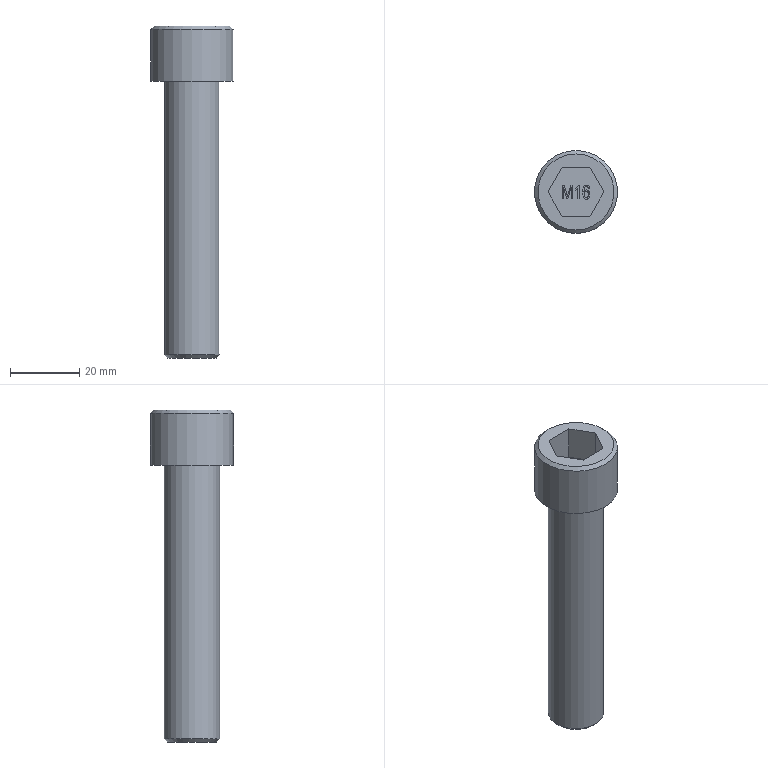Part | STEP file | M16-1 | 1 solid | 46 faces | box 24 x 24 x 96 mm | volume 21566 mm3 | plane 31 | other 11 | cylinder 2 | cone 2 | commonest cylinder face diameters 16 x1 24 x1